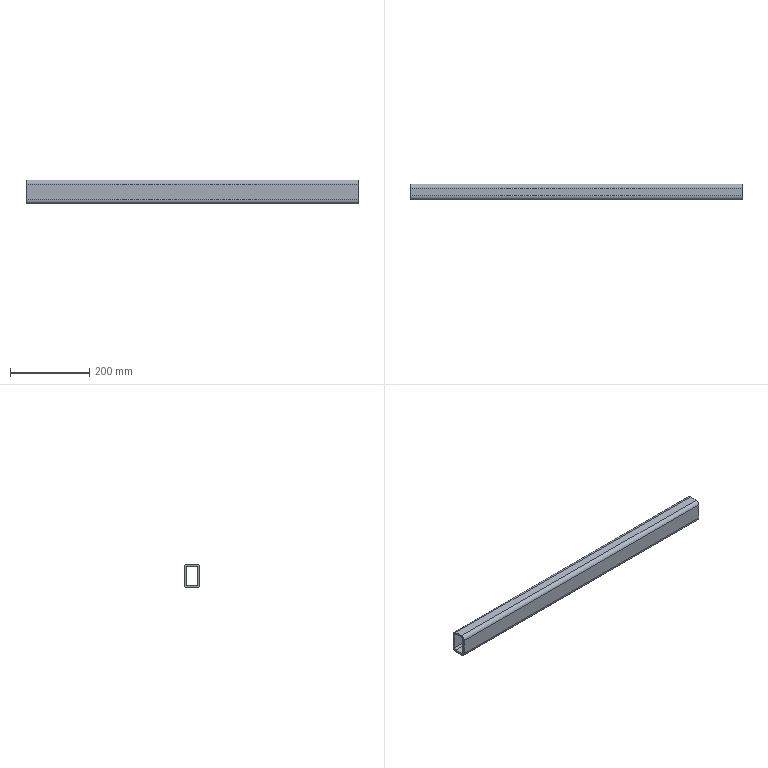Part | STEP file | frame crossmember 1--000.001--20240926 | 1 solid | 18 faces | box 837 x 40 x 60 mm | volume 699413 mm3 | plane 10 | cylinder 8 | commonest cylinder face diameters 10 x4 20 x4